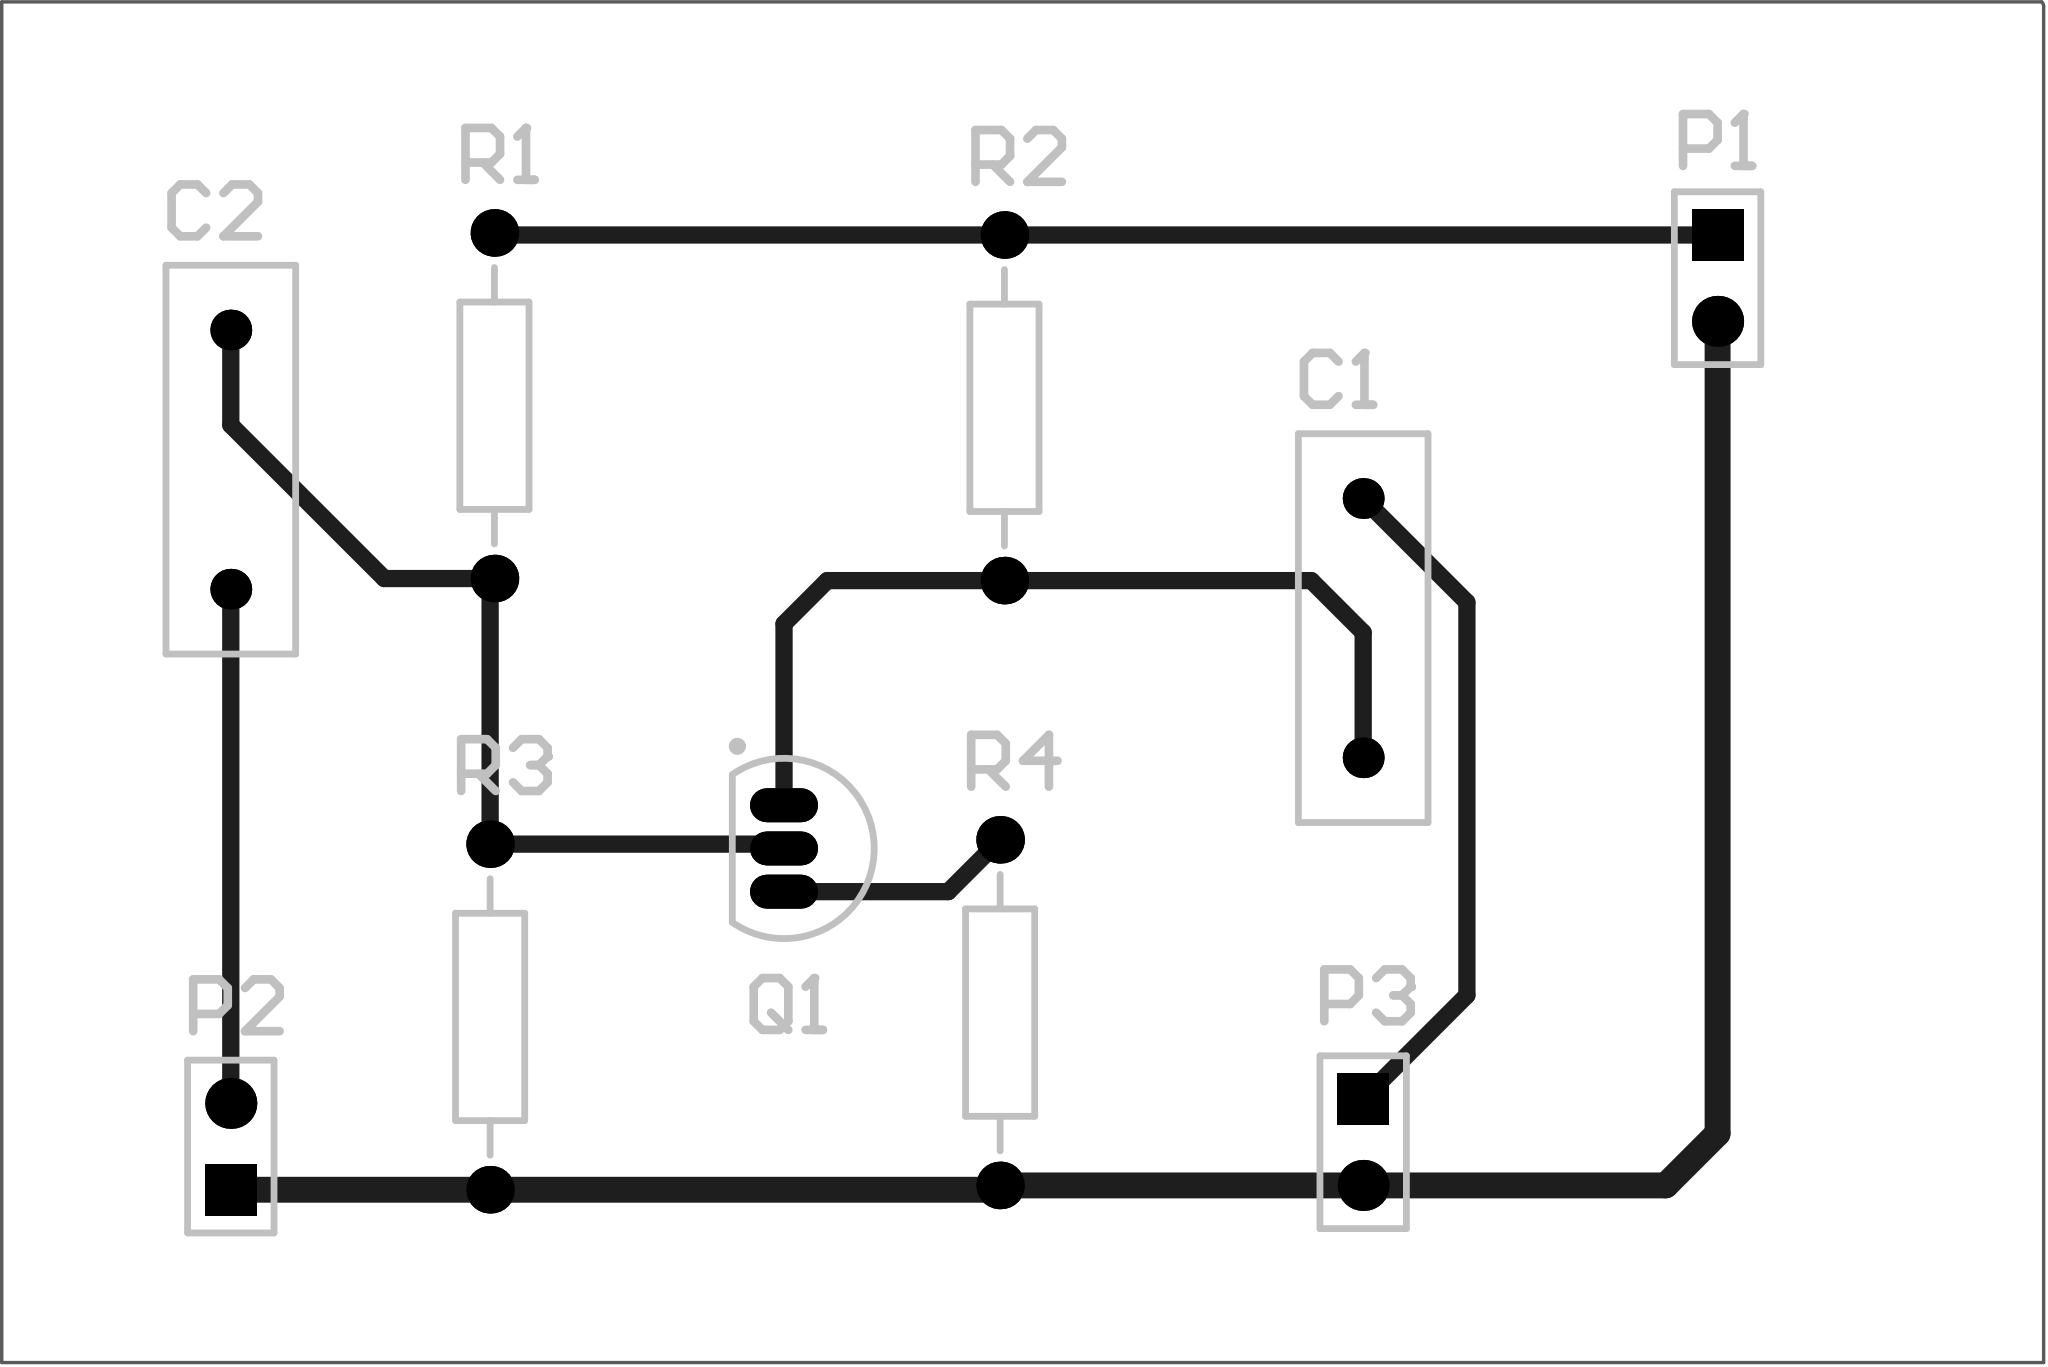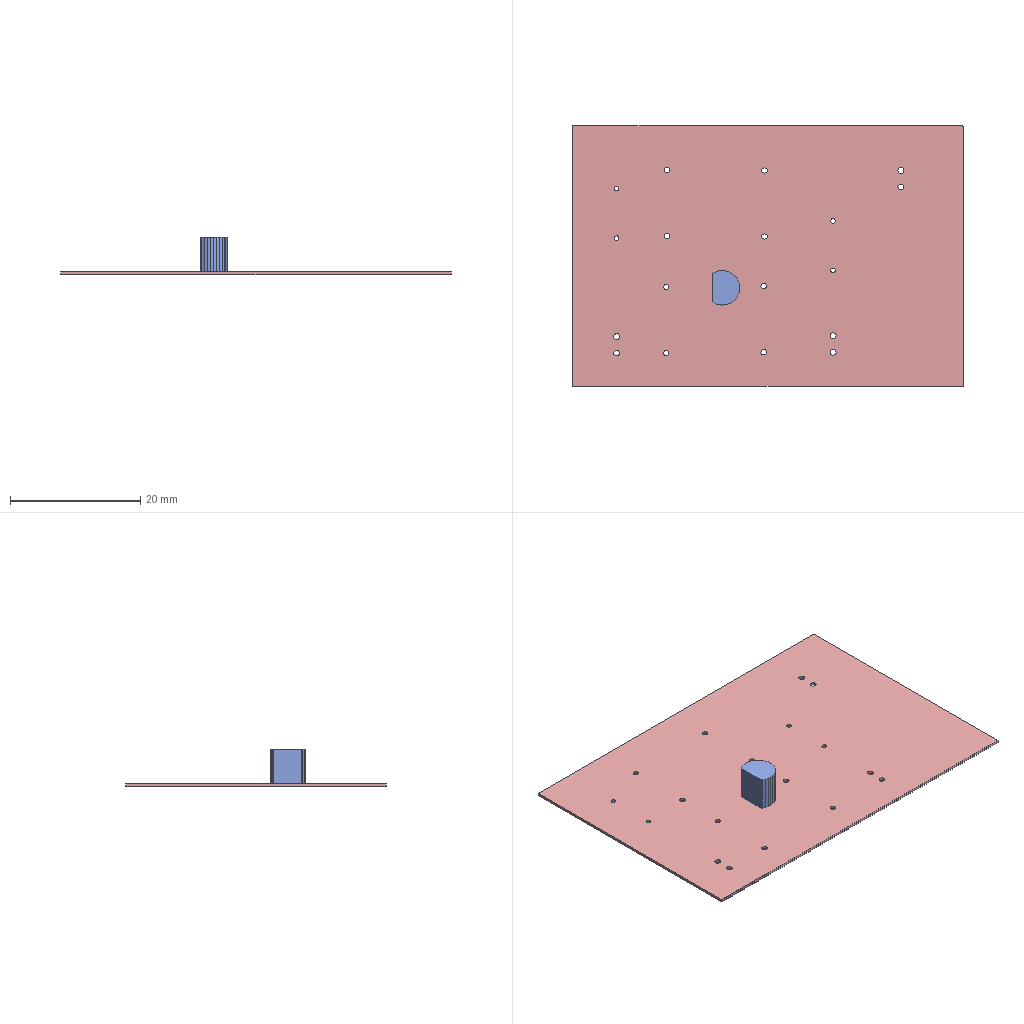Circuit board layout | Altium Designer | box 60 x 40 x 5.7 mm
Layer stack:
# Altium Designer layer stack of  (unit mm; dielectric type: 0 none, 1 core, 2 prepreg, 3 surface material)
index,name,kind,layer,copper_thickness_mm,dielectric_type,dielectric_thickness_mm,dielectric_material,dielectric_constant
0,Top Paste,other,,,,,,
1,Top Overlay,other,,,,,,
2,Top Solder,dielectric,,,3,0.0102,Solder Resist,3.5
3,Top Layer,copper,Top Layer,0.0356,,,,
4,Dielectric 1,dielectric,,,0,0.32,FR-4,4.8
5,Bottom Layer,copper,Bottom Layer,0.0356,,,,
6,Bottom Solder,dielectric,,,3,0.0102,Solder Resist,3.5
7,Bottom Overlay,other,,,,,,
8,Bottom Paste,other,,,,,,
# drill layer pairs: low layer,high layer
drill_pair,Top Layer,Bottom Layer
Part placement:
Designator,Comment,Layer,Footprint,Center-X(mm),Center-Y(mm),Rotation
R4,1K,TopLayer,AXIAL-0.4,54.737,35.687,90
R3,1K,TopLayer,AXIAL-0.4,39.751,35.56,90
R2,1K,TopLayer,AXIAL-0.4,54.864,53.467,90
R1,1K,TopLayer,AXIAL-0.4,39.878,53.527,90
Q1,NPN,TopLayer,TO-226-AA,48.387,40.513,180
P3,Header 2,TopLayer,HDR1X2,65.405,31.877,270
P2,Header 2,TopLayer,HDR1X2,32.131,31.75,90
P1,Header 2,TopLayer,HDR1X2,75.819,57.277,270
C2,100pF,TopLayer,RAD-0.3,32.131,51.943,90
C1,100pF,TopLayer,RAD-0.3,65.405,46.99,90
Pad and via stacks:
# Altium Designer via and pad stacks of  (unit mm). Each distinct definition once, with the count of objects using it.
# via: kind,start_layer,end_layer,hole_mm,diameter_mm,mode(0 simple;1 top-mid-bottom;2 full stack),diameter_per_layer,count,example_net
# pad: kind,layer,hole_mm,hole_type(0 round;1 square;2 slot),plating,top_size,top_shape(1 round;2 rect;3 octagon;9 rounded rect),mid_size,bottom_size,mode,footprint,size_per_layer,count,example
pad,Multi-Layer,0.9,0,plated,1.5x1.5,2,1.5x1.5,1.5x1.5,0,HDR1X2,,3,P1.1
pad,Multi-Layer,0.9,0,plated,1.5x1.5,1,1.5x1.5,1.5x1.5,0,HDR1X2,,3,P1.2
pad,Multi-Layer,0.85,0,plated,1.4x1.4,1,1.4x1.4,1.4x1.4,0,AXIAL-0.4,,8,R2.1
pad,Multi-Layer,0.7,0,plated,1.2x1.2,1,1.2x1.2,1.2x1.2,0,RAD-0.3,,4,C1.2
pad,Multi-Layer,0.9,0,plated,2x1,1,2x1,2x1,0,TO-226-AA,,3,Q1.1
Design rules, without the lines most boards share:
# Altium Designer design rules of  (exported by Altium Designer, unit mm)
# columns: name | kind | enabled | priority | scope1 | scope2 | descriptor | typed fields (field=value)
HoleToHoleClearance | 52 | enabled | 1 | All | All | Hole To Hole Clearance (Gap=10mil) (All),(All) | gap=0.254
DiffPairsRouting | 51 | enabled | 1 | All | All | Differential Pairs Uncoupled Length using the Gap Constraints (Min=10mil) (Max=10mil) (Prefered=10mil)  and Width Constraints (Min=15mil) (Max=15mil) (Prefered=15mil) (All) |
SolderMaskExpansion | 13 | enabled | 1 | All | All | Solder Mask Expansion (Expansion =4mil) (All) | expansion=0.1016
PasteMaskExpansion | 14 | enabled | 1 | All | All | Paste Mask Expansion (Expansion =0mil) (All) | expansion=0
RoutingVias | 11 | enabled | 1 | All | All | Routing Via (MinHoleWidth=28mil) (MaxHoleWidth=28mil) (PreferredHoleWidth=28mil) (MinWidth=50mil) (MaxWidth=50mil) (PreferedWidth=50mil) (All) | via_min_hole=0.7112 via_max_hole=0.7112 via_preferred_diameter=1.27 via_preferred_hole=0.7112
Width | 2 | enabled | 1 | All | All | Width Constraint (Min=10mil) (Max=21850.394mil) (Preferred=10mil) (All) |
PolygonConnect | 20 | enabled | 1 | All | All | Polygon Connect Rule(Relief Connect )(Conductor Width=10mil) (Relief Angle=90 Angle) (Entries=4) (Air Gap Width=10mil) (All),(All) | connect_style(0=relief,1=direct,2=none)=0 relief_conductor_width=0.254 relief_entries=4
PlaneConnect | 6 | enabled | 1 | All | All | Power Plane Connect Rule(Relief Connect )(Expansion=20mil) (Conductor Width=10mil) (Air Gap=10mil) (Entries=4) (All) | relief_conductor_width=0.254 relief_entries=4 relief_expansion=0.508
Clearance | 0 | enabled | 1 | All | All | Clearance Constraint (Gap=10mil) (All),(All) | gap=0.254